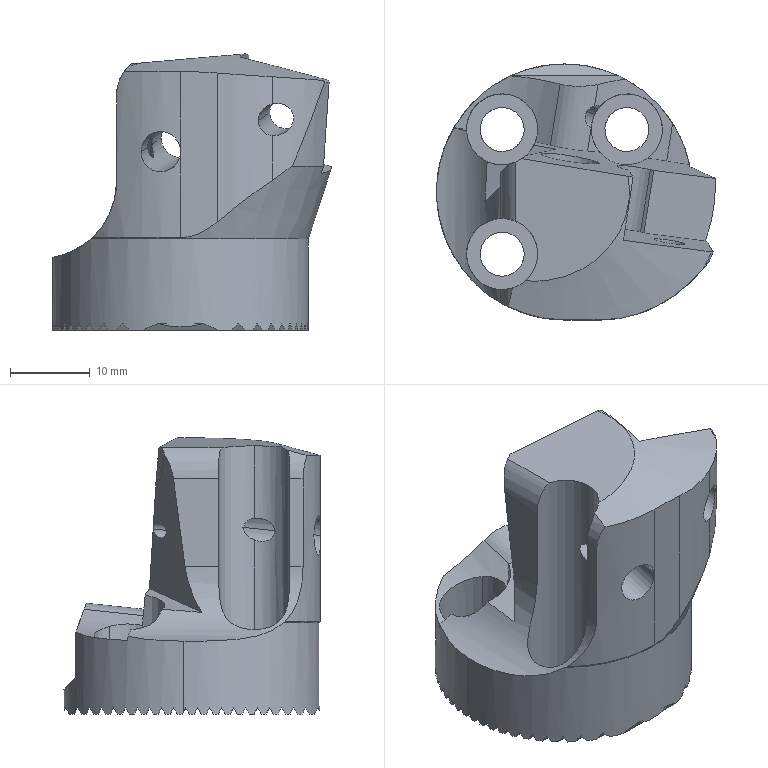Part | 1 solid | 190 faces | volume 13894 mm3 | plane 143 | cylinder 42 | cone 4 | torus 1 | commonest cylinder face diameters 8.9 x7 5.5 x6 4 x4 34 x3 2 x2 3 x2